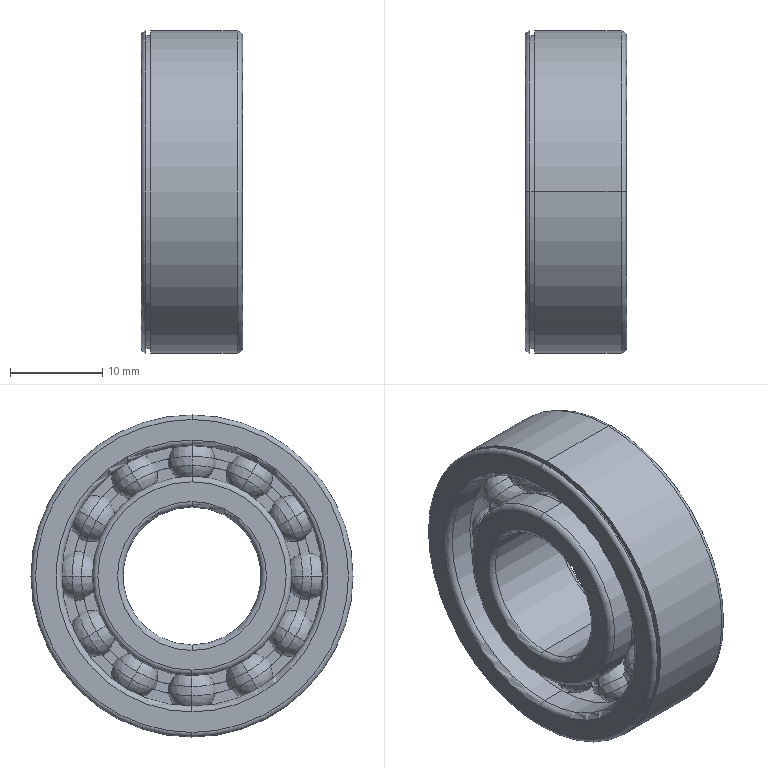Part | SolidWorks | features Revolution 5, CirPattern 2, RevCut 2, RefAxis 1 | 15 solids | 170 faces | box 11 x 35 x 35 mm | volume 6458 mm3 | cylinder 64 | sphere 52 | plane 32 | torus 22 | commonest cylinder face diameters 24 x23 26 x23 21.667 x4 28.333 x4 15 x2 20.467 x2